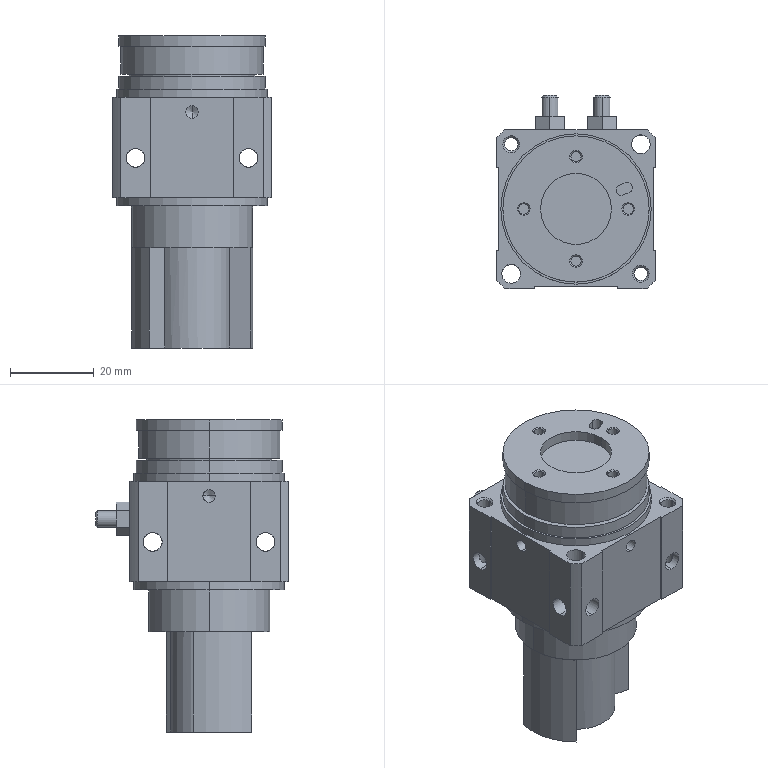Part | STEP file | MDSUB1-180S (0) | 1 solid | 187 faces | box 38 x 46.2 x 74.71 mm | volume 62029 mm3 | cylinder 97 | plane 60 | cone 30 | commonest cylinder face diameters 4.5 x38 2.46 x12 3 x6 3.24 x6 18.5 x5 29 x5